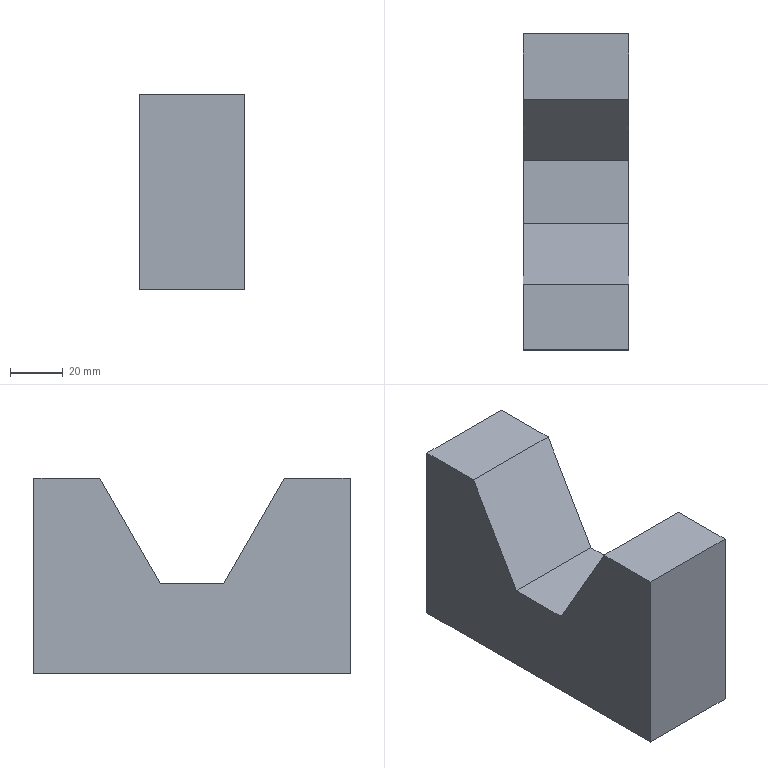Part | NX | 1 solid | 13 faces | box 40 x 120 x 74.319 mm | volume 278660 mm3 | plane 10 | cone 2 | cylinder 1 | commonest cylinder face diameters 17.5 x1
STEP:
#1=CARTESIAN_POINT('',(0.,-60.,83.063));
#2=VERTEX_POINT('',#1);
#3=CARTESIAN_POINT('',(0.,-60.,8.743));
#4=VERTEX_POINT('',#3);
#5=CARTESIAN_POINT('',(0.,-60.,83.063));
#6=DIRECTION('',(0.,0.,-1.));
#7=VECTOR('',#6,1.);
#8=LINE('',#5,#7);
#9=EDGE_CURVE('',#2,#4,#8,.T.);
#10=ORIENTED_EDGE('',*,*,#9,.T.);
#11=CARTESIAN_POINT('',(40.,-60.,8.743));
#12=VERTEX_POINT('',#11);
#13=CARTESIAN_POINT('',(40.,-60.,8.743));
#14=DIRECTION('',(-1.,0.,0.));
#15=VECTOR('',#14,1.);
#16=LINE('',#13,#15);
#17=EDGE_CURVE('',#12,#4,#16,.T.);
#18=ORIENTED_EDGE('',*,*,#17,.F.);
#19=CARTESIAN_POINT('',(40.,-60.,83.063));
#20=VERTEX_POINT('',#19);
#21=CARTESIAN_POINT('',(40.,-60.,83.063));
#22=DIRECTION('',(0.,0.,-1.));
#23=VECTOR('',#22,1.);
#24=LINE('',#21,#23);
#25=EDGE_CURVE('',#20,#12,#24,.T.);
#26=ORIENTED_EDGE('',*,*,#25,.F.);
#27=CARTESIAN_POINT('',(40.,-60.,83.063));
#28=DIRECTION('',(-1.,0.,0.));
#29=VECTOR('',#28,1.);
#30=LINE('',#27,#29);
#31=EDGE_CURVE('',#20,#2,#30,.T.);
#32=ORIENTED_EDGE('',*,*,#31,.T.);
#33=EDGE_LOOP('',(#10,#18,#26,#32));
#34=FACE_OUTER_BOUND('',#33,.T.);
#35=CARTESIAN_POINT('',(40.,-60.,83.063));
#36=DIRECTION('',(0.,1.,0.));
#37=DIRECTION('',(0.,0.,-1.));
#38=AXIS2_PLACEMENT_3D('',#35,#36,#37);
#39=PLANE('',#38);
#40=ADVANCED_FACE('',(#34),#39,.F.);
#41=CARTESIAN_POINT('',(30.,0.,8.743));
#42=VERTEX_POINT('',#41);
#43=CARTESIAN_POINT('',(20.,0.,8.743));
#44=DIRECTION('',(0.,0.,1.));
#45=DIRECTION('',(1.,0.,0.));
#46=AXIS2_PLACEMENT_3D('',#43,#44,#45);
#47=CIRCLE('',#46,10.);
#48=EDGE_CURVE('',#42,#42,#47,.T.);
#49=ORIENTED_EDGE('',*,*,#48,.T.);
#50=EDGE_LOOP('',(#49));
#51=FACE_BOUND('',#50,.T.);
#52=CARTESIAN_POINT('',(0.,60.,8.743));
#53=VERTEX_POINT('',#52);
#54=CARTESIAN_POINT('',(0.,-60.,8.743));
#55=DIRECTION('',(0.,1.,0.));
#56=VECTOR('',#55,1.);
#57=LINE('',#54,#56);
#58=EDGE_CURVE('',#4,#53,#57,.T.);
#59=ORIENTED_EDGE('',*,*,#58,.T.);
#60=CARTESIAN_POINT('',(40.,60.,8.743));
#61=VERTEX_POINT('',#60);
#62=CARTESIAN_POINT('',(40.,60.,8.743));
#63=DIRECTION('',(-1.,0.,0.));
#64=VECTOR('',#63,1.);
#65=LINE('',#62,#64);
#66=EDGE_CURVE('',#61,#53,#65,.T.);
#67=ORIENTED_EDGE('',*,*,#66,.F.);
#68=CARTESIAN_POINT('',(40.,-60.,8.743));
#69=DIRECTION('',(0.,1.,0.));
#70=VECTOR('',#69,1.);
#71=LINE('',#68,#70);
#72=EDGE_CURVE('',#12,#61,#71,.T.);
#73=ORIENTED_EDGE('',*,*,#72,.F.);
#74=ORIENTED_EDGE('',*,*,#17,.T.);
#75=EDGE_LOOP('',(#59,#67,#73,#74));
#76=FACE_BOUND('',#75,.T.);
#77=CARTESIAN_POINT('',(40.,-60.,8.743));
#78=DIRECTION('',(0.,0.,1.));
#79=DIRECTION('',(-1.,0.,0.));
#80=AXIS2_PLACEMENT_3D('',#77,#78,#79);
#81=PLANE('',#80);
#82=ADVANCED_FACE('',(#51,#76),#81,.F.);
#83=CARTESIAN_POINT('',(0.,60.,83.063));
#84=VERTEX_POINT('',#83);
#85=CARTESIAN_POINT('',(0.,60.,8.743));
#86=DIRECTION('',(0.,0.,1.));
#87=VECTOR('',#86,1.);
#88=LINE('',#85,#87);
#89=EDGE_CURVE('',#53,#84,#88,.T.);
#90=ORIENTED_EDGE('',*,*,#89,.T.);
#91=CARTESIAN_POINT('',(40.,60.,83.063));
#92=VERTEX_POINT('',#91);
#93=CARTESIAN_POINT('',(40.,60.,83.063));
#94=DIRECTION('',(-1.,0.,0.));
#95=VECTOR('',#94,1.);
#96=LINE('',#93,#95);
#97=EDGE_CURVE('',#92,#84,#96,.T.);
#98=ORIENTED_EDGE('',*,*,#97,.F.);
#99=CARTESIAN_POINT('',(40.,60.,8.743));
#100=DIRECTION('',(0.,0.,1.));
#101=VECTOR('',#100,1.);
#102=LINE('',#99,#101);
#103=EDGE_CURVE('',#61,#92,#102,.T.);
#104=ORIENTED_EDGE('',*,*,#103,.F.);
#105=ORIENTED_EDGE('',*,*,#66,.T.);
#106=EDGE_LOOP('',(#90,#98,#104,#105));
#107=FACE_OUTER_BOUND('',#106,.T.);
#108=CARTESIAN_POINT('',(40.,60.,8.743));
#109=DIRECTION('',(0.,-1.,0.));
#110=DIRECTION('',(0.,0.,1.));
#111=AXIS2_PLACEMENT_3D('',#108,#109,#110);
#112=PLANE('',#111);
#113=ADVANCED_FACE('',(#107),#112,.F.);
#114=CARTESIAN_POINT('',(0.,35.,83.063));
#115=VERTEX_POINT('',#114);
#116=CARTESIAN_POINT('',(0.,60.,83.063));
#117=DIRECTION('',(0.,-1.,0.));
#118=VECTOR('',#117,1.);
#119=LINE('',#116,#118);
#120=EDGE_CURVE('',#84,#115,#119,.T.);
#121=ORIENTED_EDGE('',*,*,#120,.T.);
#122=CARTESIAN_POINT('',(40.,35.,83.063));
#123=VERTEX_POINT('',#122);
#124=CARTESIAN_POINT('',(40.,35.,83.063));
#125=DIRECTION('',(-1.,0.,0.));
#126=VECTOR('',#125,1.);
#127=LINE('',#124,#126);
#128=EDGE_CURVE('',#123,#115,#127,.T.);
#129=ORIENTED_EDGE('',*,*,#128,.F.);
#130=CARTESIAN_POINT('',(40.,60.,83.063));
#131=DIRECTION('',(0.,-1.,0.));
#132=VECTOR('',#131,1.);
#133=LINE('',#130,#132);
#134=EDGE_CURVE('',#92,#123,#133,.T.);
#135=ORIENTED_EDGE('',*,*,#134,.F.);
#136=ORIENTED_EDGE('',*,*,#97,.T.);
#137=EDGE_LOOP('',(#121,#129,#135,#136));
#138=FACE_OUTER_BOUND('',#137,.T.);
#139=CARTESIAN_POINT('',(40.,60.,83.063));
#140=DIRECTION('',(0.,0.,-1.));
#141=DIRECTION('',(0.,-1.,0.));
#142=AXIS2_PLACEMENT_3D('',#139,#140,#141);
#143=PLANE('',#142);
#144=ADVANCED_FACE('',(#138),#143,.F.);
#145=CARTESIAN_POINT('',(0.,12.,43.063));
#146=VERTEX_POINT('',#145);
#147=CARTESIAN_POINT('',(0.,35.,83.063));
#148=DIRECTION('',(0.,-0.4985,-0.8669));
#149=VECTOR('',#148,1.);
#150=LINE('',#147,#149);
#151=EDGE_CURVE('',#115,#146,#150,.T.);
#152=ORIENTED_EDGE('',*,*,#151,.T.);
#153=CARTESIAN_POINT('',(40.,12.,43.063));
#154=VERTEX_POINT('',#153);
#155=CARTESIAN_POINT('',(40.,12.,43.063));
#156=DIRECTION('',(-1.,0.,0.));
#157=VECTOR('',#156,1.);
#158=LINE('',#155,#157);
#159=EDGE_CURVE('',#154,#146,#158,.T.);
#160=ORIENTED_EDGE('',*,*,#159,.F.);
#161=CARTESIAN_POINT('',(40.,35.,83.063));
#162=DIRECTION('',(0.,-0.4985,-0.8669));
#163=VECTOR('',#162,1.);
#164=LINE('',#161,#163);
#165=EDGE_CURVE('',#123,#154,#164,.T.);
#166=ORIENTED_EDGE('',*,*,#165,.F.);
#167=ORIENTED_EDGE('',*,*,#128,.T.);
#168=EDGE_LOOP('',(#152,#160,#166,#167));
#169=FACE_OUTER_BOUND('',#168,.T.);
#170=CARTESIAN_POINT('',(40.,35.,83.063));
#171=DIRECTION('',(0.,0.8669,-0.4985));
#172=DIRECTION('',(0.,-0.4985,-0.8669));
#173=AXIS2_PLACEMENT_3D('',#170,#171,#172);
#174=PLANE('',#173);
#175=ADVANCED_FACE('',(#169),#174,.F.);
#176=CARTESIAN_POINT('',(0.,-12.,43.063));
#177=VERTEX_POINT('',#176);
#178=CARTESIAN_POINT('',(0.,12.,43.063));
#179=DIRECTION('',(0.,-1.,0.));
#180=VECTOR('',#179,1.);
#181=LINE('',#178,#180);
#182=EDGE_CURVE('',#146,#177,#181,.T.);
#183=ORIENTED_EDGE('',*,*,#182,.T.);
#184=CARTESIAN_POINT('',(40.,-12.,43.063));
#185=VERTEX_POINT('',#184);
#186=CARTESIAN_POINT('',(40.,-12.,43.063));
#187=DIRECTION('',(-1.,0.,0.));
#188=VECTOR('',#187,1.);
#189=LINE('',#186,#188);
#190=EDGE_CURVE('',#185,#177,#189,.T.);
#191=ORIENTED_EDGE('',*,*,#190,.F.);
#192=CARTESIAN_POINT('',(40.,12.,43.063));
#193=DIRECTION('',(0.,-1.,0.));
#194=VECTOR('',#193,1.);
#195=LINE('',#192,#194);
#196=EDGE_CURVE('',#154,#185,#195,.T.);
#197=ORIENTED_EDGE('',*,*,#196,.F.);
#198=ORIENTED_EDGE('',*,*,#159,.T.);
#199=EDGE_LOOP('',(#183,#191,#197,#198));
#200=FACE_OUTER_BOUND('',#199,.T.);
#201=CARTESIAN_POINT('',(40.,12.,43.063));
#202=DIRECTION('',(0.,0.,-1.));
#203=DIRECTION('',(1.,0.,0.));
#204=AXIS2_PLACEMENT_3D('',#201,#202,#203);
#205=PLANE('',#204);
#206=ADVANCED_FACE('',(#200),#205,.F.);
#207=CARTESIAN_POINT('',(0.,-35.,83.063));
#208=VERTEX_POINT('',#207);
#209=CARTESIAN_POINT('',(0.,-12.,43.063));
#210=DIRECTION('',(0.,-0.4985,0.8669));
#211=VECTOR('',#210,1.);
#212=LINE('',#209,#211);
#213=EDGE_CURVE('',#177,#208,#212,.T.);
#214=ORIENTED_EDGE('',*,*,#213,.T.);
#215=CARTESIAN_POINT('',(40.,-35.,83.063));
#216=VERTEX_POINT('',#215);
#217=CARTESIAN_POINT('',(40.,-35.,83.063));
#218=DIRECTION('',(-1.,0.,0.));
#219=VECTOR('',#218,1.);
#220=LINE('',#217,#219);
#221=EDGE_CURVE('',#216,#208,#220,.T.);
#222=ORIENTED_EDGE('',*,*,#221,.F.);
#223=CARTESIAN_POINT('',(40.,-12.,43.063));
#224=DIRECTION('',(0.,-0.4985,0.8669));
#225=VECTOR('',#224,1.);
#226=LINE('',#223,#225);
#227=EDGE_CURVE('',#185,#216,#226,.T.);
#228=ORIENTED_EDGE('',*,*,#227,.F.);
#229=ORIENTED_EDGE('',*,*,#190,.T.);
#230=EDGE_LOOP('',(#214,#222,#228,#229));
#231=FACE_OUTER_BOUND('',#230,.T.);
#232=CARTESIAN_POINT('',(40.,-12.,43.063));
#233=DIRECTION('',(0.,-0.8669,-0.4985));
#234=DIRECTION('',(0.,-0.4985,0.8669));
#235=AXIS2_PLACEMENT_3D('',#232,#233,#234);
#236=PLANE('',#235);
#237=ADVANCED_FACE('',(#231),#236,.F.);
#238=CARTESIAN_POINT('',(0.,-35.,83.063));
#239=DIRECTION('',(0.,-1.,0.));
#240=VECTOR('',#239,1.);
#241=LINE('',#238,#240);
#242=EDGE_CURVE('',#208,#2,#241,.T.);
#243=ORIENTED_EDGE('',*,*,#242,.T.);
#244=ORIENTED_EDGE('',*,*,#31,.F.);
#245=CARTESIAN_POINT('',(40.,-35.,83.063));
#246=DIRECTION('',(0.,-1.,0.));
#247=VECTOR('',#246,1.);
#248=LINE('',#245,#247);
#249=EDGE_CURVE('',#216,#20,#248,.T.);
#250=ORIENTED_EDGE('',*,*,#249,.F.);
#251=ORIENTED_EDGE('',*,*,#221,.T.);
#252=EDGE_LOOP('',(#243,#244,#250,#251));
#253=FACE_OUTER_BOUND('',#252,.T.);
#254=CARTESIAN_POINT('',(40.,-35.,83.063));
#255=DIRECTION('',(0.,0.,-1.));
#256=DIRECTION('',(0.,-1.,0.));
#257=AXIS2_PLACEMENT_3D('',#254,#255,#256);
#258=PLANE('',#257);
#259=ADVANCED_FACE('',(#253),#258,.F.);
#260=ORIENTED_EDGE('',*,*,#25,.T.);
#261=ORIENTED_EDGE('',*,*,#72,.T.);
#262=ORIENTED_EDGE('',*,*,#103,.T.);
#263=ORIENTED_EDGE('',*,*,#134,.T.);
#264=ORIENTED_EDGE('',*,*,#165,.T.);
#265=ORIENTED_EDGE('',*,*,#196,.T.);
#266=ORIENTED_EDGE('',*,*,#227,.T.);
#267=ORIENTED_EDGE('',*,*,#249,.T.);
#268=EDGE_LOOP('',(#260,#261,#262,#263,#264,#265,#266,#267));
#269=FACE_OUTER_BOUND('',#268,.T.);
#270=CARTESIAN_POINT('',(40.,0.,0.));
#271=DIRECTION('',(1.,0.,0.));
#272=DIRECTION('',(0.,0.,1.));
#273=AXIS2_PLACEMENT_3D('',#270,#271,#272);
#274=PLANE('',#273);
#275=ADVANCED_FACE('',(#269),#274,.T.);
#276=ORIENTED_EDGE('',*,*,#9,.F.);
#277=ORIENTED_EDGE('',*,*,#242,.F.);
#278=ORIENTED_EDGE('',*,*,#213,.F.);
#279=ORIENTED_EDGE('',*,*,#182,.F.);
#280=ORIENTED_EDGE('',*,*,#151,.F.);
#281=ORIENTED_EDGE('',*,*,#120,.F.);
#282=ORIENTED_EDGE('',*,*,#89,.F.);
#283=ORIENTED_EDGE('',*,*,#58,.F.);
#284=EDGE_LOOP('',(#276,#277,#278,#279,#280,#281,#282,#283));
#285=FACE_OUTER_BOUND('',#284,.T.);
#286=CARTESIAN_POINT('',(0.,0.,0.));
#287=DIRECTION('',(1.,0.,0.));
#288=DIRECTION('',(0.,0.,1.));
#289=AXIS2_PLACEMENT_3D('',#286,#287,#288);
#290=PLANE('',#289);
#291=ADVANCED_FACE('',(#285),#290,.F.);
#292=CARTESIAN_POINT('',(28.75,0.,18.743));
#293=VERTEX_POINT('',#292);
#294=CARTESIAN_POINT('',(20.,0.,18.743));
#295=DIRECTION('',(0.,0.,-1.));
#296=DIRECTION('',(1.,0.,0.));
#297=AXIS2_PLACEMENT_3D('',#294,#295,#296);
#298=CIRCLE('',#297,8.75);
#299=EDGE_CURVE('',#293,#293,#298,.T.);
#300=ORIENTED_EDGE('',*,*,#299,.T.);
#301=EDGE_LOOP('',(#300));
#302=FACE_BOUND('',#301,.T.);
#303=CARTESIAN_POINT('',(20.,0.,24.001));
#304=VERTEX_POINT('',#303);
#305=VERTEX_LOOP('',#304);
#306=FACE_BOUND('',#305,.T.);
#307=CARTESIAN_POINT('',(20.,0.,18.743));
#308=DIRECTION('',(0.,0.,-1.));
#309=DIRECTION('',(1.,0.,0.));
#310=AXIS2_PLACEMENT_3D('',#307,#308,#309);
#311=CONICAL_SURFACE('',#310,8.75,59.);
#312=ADVANCED_FACE('',(#302,#306),#311,.F.);
#313=CARTESIAN_POINT('',(28.75,0.,9.993));
#314=VERTEX_POINT('',#313);
#315=CARTESIAN_POINT('',(20.,0.,9.993));
#316=DIRECTION('',(0.,0.,-1.));
#317=DIRECTION('',(1.,0.,0.));
#318=AXIS2_PLACEMENT_3D('',#315,#316,#317);
#319=CIRCLE('',#318,8.75);
#320=EDGE_CURVE('',#314,#314,#319,.T.);
#321=ORIENTED_EDGE('',*,*,#320,.T.);
#322=EDGE_LOOP('',(#321));
#323=FACE_BOUND('',#322,.T.);
#324=ORIENTED_EDGE('',*,*,#299,.F.);
#325=EDGE_LOOP('',(#324));
#326=FACE_BOUND('',#325,.T.);
#327=CARTESIAN_POINT('',(20.,0.,8.743));
#328=DIRECTION('',(0.,0.,1.));
#329=DIRECTION('',(-1.,0.,0.));
#330=AXIS2_PLACEMENT_3D('',#327,#328,#329);
#331=CYLINDRICAL_SURFACE('',#330,8.75);
#332=ADVANCED_FACE('',(#323,#326),#331,.F.);
#333=ORIENTED_EDGE('',*,*,#320,.F.);
#334=EDGE_LOOP('',(#333));
#335=FACE_BOUND('',#334,.T.);
#336=ORIENTED_EDGE('',*,*,#48,.F.);
#337=EDGE_LOOP('',(#336));
#338=FACE_BOUND('',#337,.T.);
#339=CARTESIAN_POINT('',(20.,0.,8.743));
#340=DIRECTION('',(0.,0.,-1.));
#341=DIRECTION('',(1.,0.,0.));
#342=AXIS2_PLACEMENT_3D('',#339,#340,#341);
#343=CONICAL_SURFACE('',#342,10.,45.);
#344=ADVANCED_FACE('',(#335,#338),#343,.F.);
#345=CLOSED_SHELL('',(#40,#82,#113,#144,#175,#206,#237,#259,#275,#291,#312,#332,#344));
#346=MANIFOLD_SOLID_BREP('',#345);
#347=(LENGTH_UNIT()NAMED_UNIT(*)SI_UNIT(.MILLI.,.METRE.));
#348=UNCERTAINTY_MEASURE_WITH_UNIT(LENGTH_MEASURE(0.00002),#347,'','');
#349=(NAMED_UNIT(*)PLANE_ANGLE_UNIT()SI_UNIT($,.RADIAN.));
#350=PLANE_ANGLE_MEASURE_WITH_UNIT(PLANE_ANGLE_MEASURE(0.01745),#349);
#351=DIMENSIONAL_EXPONENTS(0.,0.,0.,0.,0.,0.,0.);
#352=(CONVERSION_BASED_UNIT('DEGREE',#350)NAMED_UNIT(#351)PLANE_ANGLE_UNIT());
#353=(NAMED_UNIT(*)SI_UNIT($,.STERADIAN.)SOLID_ANGLE_UNIT());
#354=(GEOMETRIC_REPRESENTATION_CONTEXT(3)GLOBAL_UNCERTAINTY_ASSIGNED_CONTEXT((#348))GLOBAL_UNIT_ASSIGNED_CONTEXT((#347,#352,#353))REPRESENTATION_CONTEXT('',''));
#355=ADVANCED_BREP_SHAPE_REPRESENTATION('',(#346),#354);